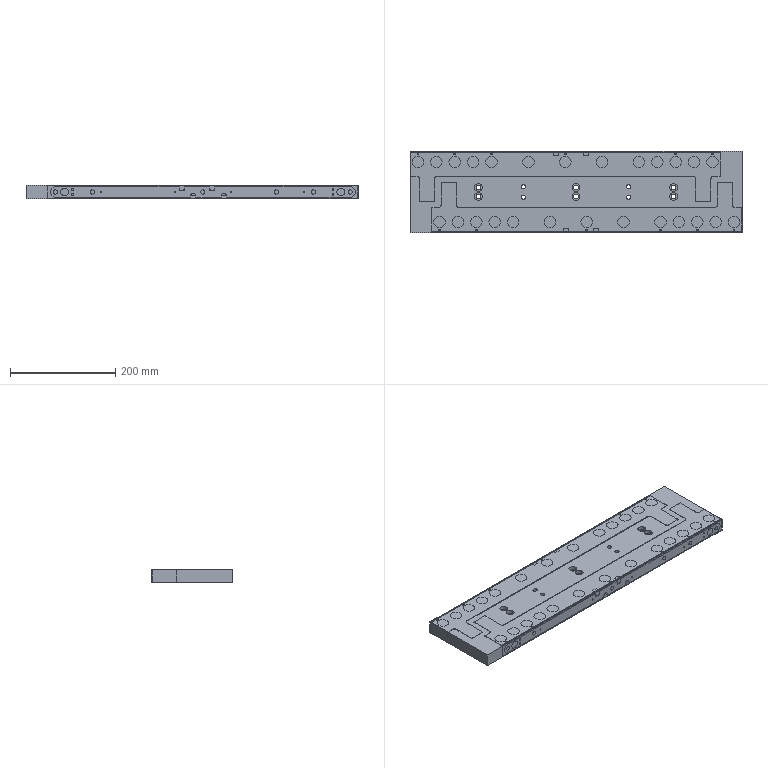NC program | NX | posted with a generic post | part box 631 x 154 x 25 mm
Whole program:
N10 G17 G21 G94 G90
(DRILLING_COPY_1_COPY , TOOL : D6A45)
N12 T07 M6
N14 G54
N16 G17 G0 G90 X280. Y0. B0. C0. S3000 M3
N18 G43 Z30. H7
N20 G94 G81 G98 Z-2.1 F200. R3.
N22 X262.5
N24 X247.5 Y-4.5
N26 Y4.5
N28 X210. Y0.
N30 X0.
N32 X-140.
N34 X-210.
N36 X-247.5 Y4.5
N38 Y-4.5
N40 X-262.5 Y0.
N42 X-280.
N44 G80
N46 G0 X-280. Y0. Z30.
(DRILLING_COPY_1_COPY_COPY , TOOL : D6A45)
N48 X-193.
N50 G81 Z-1.6 F200. R3.
N52 X-53.
N54 X53.
N56 X193.
N58 G80
N60 G0 X193. Y0. Z30.
N62 M5
(DRILLING_COPY_2_COPY_1 , TOOL : 3.3ZT)
N64 T13 M6
N66 G54
N68 G17 G0 G90 X-247.5 Y-4.5 B0. C0. S2000 M3
N70 G43 Z30. H13
N72 G94 G83 G98 Z-10.991 F100. Q2. R3.
N74 Y4.5
N76 X247.5
N78 Y-4.5
N80 G80
N82 G0 X247.5 Y-4.5 Z30.
N84 M5
(DRILLING_COPY_2_COPY_1_COPY , TOOL : 2.5ZT)
N86 T12 M6
N88 G54
N90 G17 G0 G90 X-193. Y0. B0. C0. S2000 M3
N92 G43 Z30. H12
N94 G94 G83 G98 Z-10.751 F100. Q2. R3.
N96 X-53.
N98 X53.
N100 X193.
N102 G80
N104 G0 X193. Y0. Z30.
N106 M5
(DRILLING_COPY_2_COPY_1_COPY_COPY , TOOL : 5.5ZT)
N108 T15 M6
N110 G54
N112 G17 G0 G90 X-40. Y7.5 B0. C0. S2000 M3
N114 G43 Z30. H15
N116 G94 G83 G98 Z-51.152 F250. Q2. R3.
N118 X-18. Y-7.5
N120 X18. Y7.5
N122 X40. Y-7.5
N124 G80
N126 G0 X40. Y-7.5 Z30.
N128 M5
(DRILLING_COPY_COPY_1 , TOOL : 10.5ZT)
N130 T09 M6
N132 G54
N134 G17 G0 G90 X-262.5 Y0. B0. C0. S1000 M3
N136 G43 Z30. H9
N138 G94 G83 G98 Z-99.204 F100. Q2. R3.
N140 X262.5
N142 G80
N144 G0 X262.5 Y0. Z30.
N146 M5
(DRILLING_COPY_COPY_COPY_1 , TOOL : 7.8ZT)
N148 T17 M6
N150 G54
N152 G17 G0 G90 X-280. Y0. B0. C0. S2000 M3
N154 G43 Z30. H17
N156 G94 G83 G98 Z-16.915 F200. Q2. R3.
N158 X-210.
N160 X-140.
N162 X0.
N164 X210.
N166 X280.
N168 G80
N170 G0 X280. Y0. Z30.
N172 M5
(DRILLING_COPY_COPY_COPY_COPY , TOOL : 8.0JD)
N174 T18 M6
N176 G54
N178 G17 G0 G90 X-280. Y0. B0. C0. S1000 M3
N180 G43 Z30. H18
N182 G94 G85 G98 Z-13.572 F50. R3.
N184 X-210.
N186 X-140.
N188 X0.
N190 X210.
N192 X280.
N194 G80
N196 G0 X280. Y0. Z30.
N198 M5
(HOLE_MILLING_COPY_1_COPY , TOOL : D10)
N200 T10 M6
N202 G54
N204 G17 G0 G90 X-262.5 Y0. B0. C0. S7000 M3
N206 G43 Z30. H10
N208 Z1.
N210 G94 G3 X-263.745 Y1.245 R1.245 F1500.
N212 X-264.99 Y0. R1.245
N214 X-264.99 Y0. Z0. I2.49 J0.
N216 X-264.99 Y0. Z-1. I2.49 J0.
N218 X-264.99 Y0. Z-2. I2.49 J0.
N220 X-264.99 Y0. Z-3. I2.49 J0.
N222 X-264.99 Y0. Z-4. I2.49 J0.
N224 X-264.99 Y0. Z-5. I2.49 J0.
N226 X-264.99 Y0. Z-6. I2.49 J0.
N228 X-264.99 Y0. Z-7. I2.49 J0.
N230 X-264.99 Y0. Z-8. I2.49 J0.
N232 X-264.99 Y0. Z-9. I2.49 J0.
N234 X-264.99 Y0. Z-10. I2.49 J0.
N236 X-264.99 Y0. Z-11. I2.49 J0.
N238 X-264.99 Y0. Z-12. I2.49 J0.
N240 X-264.99 Y0. Z-13. I2.49 J0.
N242 X-264.99 Y0. Z-14. I2.49 J0.
N244 X-264.99 Y0. Z-15. I2.49 J0.
N246 X-264.99 Y0. Z-16. I2.49 J0.
N248 X-264.99 Y0. Z-17. I2.49 J0.
N250 X-264.99 Y0. Z-18. I2.49 J0.
N252 X-264.99 Y0. Z-19. I2.49 J0.
N254 X-264.99 Y0. Z-20. I2.49 J0.
N256 X-264.99 Y0. Z-21. I2.49 J0.
N258 X-264.99 Y0. Z-22. I2.49 J0.
N260 X-264.99 Y0. Z-23. I2.49 J0.
N262 X-264.99 Y0. Z-24. I2.49 J0.
N264 X-264.99 Y0. Z-25. I2.49 J0.
N266 X-264.99 Y0. Z-26. I2.49 J0.
N268 X-264.99 Y0. Z-27. I2.49 J0.
N270 X-264.99 Y0. Z-28. I2.49 J0.
N272 X-264.99 Y0. Z-29. I2.49 J0.
N274 X-264.99 Y0. Z-30. I2.49 J0.
N276 X-264.99 Y0. Z-31. I2.49 J0.
N278 X-264.99 Y0. Z-32. I2.49 J0.
N280 X-264.99 Y0. Z-33. I2.49 J0.
N282 X-264.99 Y0. Z-34. I2.49 J0.
N284 X-264.99 Y0. Z-35. I2.49 J0.
N286 X-262.5 Y-2.49 R2.49
N288 X-264.99 Y0. R-2.49
N290 X-263.745 Y-1.245 R1.245
N292 X-262.5 Y0. R1.245
N294 G0 Z30.
N296 X262.5
N298 Z1.
N300 G3 X261.255 Y1.245 R1.245
N302 X260.01 Y0. R1.245
N304 X260.01 Y0. Z0. I2.49 J0.
N306 X260.01 Y0. Z-1. I2.49 J0.
N308 X260.01 Y0. Z-2. I2.49 J0.
N310 X260.01 Y0. Z-3. I2.49 J0.
N312 X260.01 Y0. Z-4. I2.49 J0.
N314 X260.01 Y0. Z-5. I2.49 J0.
N316 X260.01 Y0. Z-6. I2.49 J0.
N318 X260.01 Y0. Z-7. I2.49 J0.
N320 X260.01 Y0. Z-8. I2.49 J0.
N322 X260.01 Y0. Z-9. I2.49 J0.
N324 X260.01 Y0. Z-10. I2.49 J0.
N326 X260.01 Y0. Z-11. I2.49 J0.
N328 X260.01 Y0. Z-12. I2.49 J0.
N330 X260.01 Y0. Z-13. I2.49 J0.
N332 X260.01 Y0. Z-14. I2.49 J0.
N334 X260.01 Y0. Z-15. I2.49 J0.
N336 X260.01 Y0. Z-16. I2.49 J0.
N338 X260.01 Y0. Z-17. I2.49 J0.
N340 X260.01 Y0. Z-18. I2.49 J0.
N342 X260.01 Y0. Z-19. I2.49 J0.
N344 X260.01 Y0. Z-20. I2.49 J0.
N346 X260.01 Y0. Z-21. I2.49 J0.
N348 X260.01 Y0. Z-22. I2.49 J0.
N350 X260.01 Y0. Z-23. I2.49 J0.
N352 X260.01 Y0. Z-24. I2.49 J0.
N354 X260.01 Y0. Z-25. I2.49 J0.
N356 X260.01 Y0. Z-26. I2.49 J0.
N358 X260.01 Y0. Z-27. I2.49 J0.
N360 X260.01 Y0. Z-28. I2.49 J0.
N362 X260.01 Y0. Z-29. I2.49 J0.
N364 X260.01 Y0. Z-30. I2.49 J0.
N366 X260.01 Y0. Z-31. I2.49 J0.
N368 X260.01 Y0. Z-32. I2.49 J0.
N370 X260.01 Y0. Z-33. I2.49 J0.
N372 X260.01 Y0. Z-34. I2.49 J0.
N374 X260.01 Y0. Z-35. I2.49 J0.
N376 X262.5 Y-2.49 R2.49
N378 X260.01 Y0. R-2.49
N380 X261.255 Y-1.245 R1.245
N382 X262.5 Y0. R1.245
N384 G0 Z30.
(ZLEVEL_PROFILE_COPY_1 , TOOL : D10)
N386 X104.274 Y15.15
N388 Z1.5
N390 G1 X151.5 Z-0.975 F1000.
N392 X280. F3000.
N394 G2 X295.15 Y0. R15.15
N396 X280. Y-15.15 R15.15
N398 G1 X45.
N400 G2 X40. Y-11.234 R5.15
N402 X35. Y-15.15 R5.15
N404 G1 X-13.
N406 G2 X-18. Y-11.234 R5.15
N408 X-23. Y-15.15 R5.15
N410 G1 X-280.
N412 G2 X-295.15 Y0. R15.15
N414 X-280. Y15.15 R15.15
N416 G1 X-45.
N418 G2 X-40.018 Y11.306 R5.15
N420 G1 X-39.992 Y11.266
N422 G2 X-35. Y15.15 R5.15
N424 G1 X13.
N426 G2 X17.978 Y11.318 R5.15
N428 X23. Y15.15 R5.15
N430 G1 X151.5
N432 X207.358 Z-1.95
N434 X280.
N436 G2 X295.15 Y0. R15.15
N438 X280. Y-15.15 R15.15
N440 G1 X45.
N442 G2 X40. Y-11.234 R5.15
N444 X35. Y-15.15 R5.15
N446 G1 X-13.
N448 G2 X-18. Y-11.234 R5.15
N450 X-23. Y-15.15 R5.15
N452 G1 X-280.
N454 G2 X-295.15 Y0. R15.15
N456 X-280. Y15.15 R15.15
N458 G1 X-45.
N460 G2 X-40.018 Y11.306 R5.15
N462 G1 X-39.992 Y11.266
N464 G2 X-35. Y15.15 R5.15
N466 G1 X13.
N468 G2 X17.978 Y11.318 R5.15
N470 X23. Y15.15 R5.15
N472 G1 X207.358
N474 Z-0.45
N476 G0 Z30.
N478 M5
(HOLE_MILLING_COPY_1_COPY_COPY , TOOL : D10JING)
N480 T11 M6
N482 G54
N484 G17 G0 G90 X-262.5 Y0. B0. C0. S7000 M3
N486 G43 Z30. H11
N488 Z1.
N490 G94 G3 X-263.75 Y1.25 R1.25 F1000.
N492 X-265. Y0. R1.25
N494 X-265. Y0. Z-4. I2.5 J0.
N496 X-265. Y0. Z-9. I2.5 J0.
N498 X-265. Y0. Z-14. I2.5 J0.
N500 X-265. Y0. Z-19. I2.5 J0.
N502 X-265. Y0. Z-24. I2.5 J0.
N504 X-265. Y0. Z-29. I2.5 J0.
N506 X-265. Y0. Z-34. I2.5 J0.
N508 X-263.273 Y-2.378 Z-35. R2.5
N510 X-260.122 Y-0.773 R2.5
N512 X-263.273 Y-2.378 R-2.5
N514 X-261.697 Y-1.575 R1.25
N516 X-262.5 Y0. R1.25
N518 G0 Z30.
N520 X262.5
N522 Z1.
N524 G3 X261.25 Y1.25 R1.25
N526 X260. Y0. R1.25
N528 X260. Y0. Z-4. I2.5 J0.
N530 X260. Y0. Z-9. I2.5 J0.
N532 X260. Y0. Z-14. I2.5 J0.
N534 X260. Y0. Z-19. I2.5 J0.
N536 X260. Y0. Z-24. I2.5 J0.
N538 X260. Y0. Z-29. I2.5 J0.
N540 X260. Y0. Z-34. I2.5 J0.
N542 X261.727 Y-2.378 Z-35. R2.5
N544 X264.878 Y-0.773 R2.5
N546 X261.727 Y-2.378 R-2.5
N548 X263.303 Y-1.575 R1.25
N550 X262.5 Y0. R1.25
N552 G0 Z30.
(ZLEVEL_PROFILE_COPY_2 , TOOL : D10JING)
N554 X149.116 Y19.
N556 Z-2.
N558 G1 X149.53 Y16.653 F1200.
N560 G3 X151.5 Y15. R2.
N562 G1 X280.
N564 G2 X295. Y0. R15.
N566 X280. Y-15. R15.
N568 G1 X45.
N570 G2 X40.047 Y-10.682 R5.
N572 X35. Y-15. R5.
N574 G1 X-13.
N576 G2 X-17.99 Y-10.312 R5.
N578 G1 X-18.013 Y-10.315
N580 X-18.011 Y-10.337
N582 G2 X-23. Y-15. R5.
N584 G1 X-280.
N586 G2 X-295. Y0. R15.
N588 X-280. Y15. R15.
N590 G1 X-45.
N592 G2 X-40.047 Y10.682 R5.
N594 X-35. Y15. R5.
N596 G1 X13.
N598 G2 X17.989 Y10.326 R5.
N600 G1 X18.014 Y10.397
N602 X18.017 Y10.411
N604 G2 X23. Y15. R5.
N606 G1 X151.5
N608 G3 X153.47 Y16.653 R2.
N610 G1 X153.884 Y19.
N612 G0 Z30.
N614 M5
(111 , TOOL : D8JING)
N616 T08 M6
N618 G54
N620 G17 G0 G90 X17.999 Y19.413 B0. C0. S7000 M3
N622 G43 Z30. H8
N624 Z0.
N626 G94 G1 Z-1. F1800.
N628 X17.394 Y17.224
N630 G3 X16.998 Y16.529 R0.8
N632 G1 X17.001 Y16.131
N634 X17. Y10.
N636 Y7.5
N638 G3 X18. Y6.5 R1.
N640 X19. Y7.5 R1.
N642 G1 Y10.
N644 X19.003 Y16.529
N646 G3 X18.603 Y17.222 R0.8
N648 G1 X17.999 Y19.413
N650 Z0.
N652 G0 X18. Y19.411 Z-1.
N654 G1 Z-2.
N656 X17.394 Y17.224
N658 G3 X16.998 Y16.529 R0.8
N660 G1 X17.001 Y16.131
N662 X17. Y10.
N664 Y7.5
N666 G3 X18. Y6.5 R1.
N668 X19. Y7.5 R1.
N670 G1 Y10.
N672 X19.003 Y16.529
N674 G3 X18.603 Y17.222 R0.8
N676 G1 X18. Y19.411
N678 Z-1.
N680 G0 X18.001 Y19.414 Z-2.
N682 G1 Z-3.
N684 X17.394 Y17.224
N686 G3 X16.998 Y16.529 R0.8
N688 G1 X17.001 Y16.131
N690 Y12.546
N692 X17. Y12.148
N694 Y7.5
N696 G3 X18. Y6.5 R1.
N698 X19. Y7.5 R1.
N700 G1 Y12.148
N702 X19.003 Y16.529
N704 G3 X18.603 Y17.222 R0.8
N706 G1 X18.001 Y19.414
N708 Z-2.
N710 G0 Z-3.
N712 G1 Z-4.
N714 X17.394 Y17.224
N716 G3 X16.999 Y16.529 R0.8
N718 G1 X17.001 Y16.131
N720 Y12.546
N722 X17. Y12.148
N724 Y7.5
N726 G3 X18. Y6.5 R1.
N728 X19. Y7.5 R1.
N730 G1 Y12.148
N732 X19.003 Y16.529
N734 G3 X18.603 Y17.222 R0.8
N736 G1 X18.001 Y19.414
N738 Z-3.
N740 G0 Z-4.
N742 G1 Z-5.
N744 X17.394 Y17.224
N746 G3 X16.999 Y16.529 R0.8
N748 G1 X17.001 Y16.131
N750 Y12.546
N752 X17. Y12.148
N754 Y7.5
N756 G3 X18. Y6.5 R1.
N758 X19. Y7.5 R1.
N760 G1 Y12.148
N762 X19.002 Y16.529
N764 G3 X18.603 Y17.222 R0.8
N766 G1 X18.001 Y19.414
N768 Z-4.
N770 G0 Y19.415 Z-5.
N772 G1 Z-6.
N774 X17.394 Y17.224
N776 G3 X16.999 Y16.529 R0.8
N778 G1 X17.002 Y16.131
N780 Y12.546
N782 X17. Y12.148
N784 Y7.5
N786 G3 X18. Y6.5 R1.
N788 X19. Y7.5 R1.
N790 G1 Y12.148
N792 X19.002 Y16.529
N794 G3 X18.603 Y17.222 R0.8
N796 G1 X18.001 Y19.415
N798 Z-5.
N800 G0 Z-6.
N802 G1 Z-7.
N804 X17.394 Y17.224
N806 G3 X16.999 Y16.529 R0.8
N808 G1 X17.002 Y16.131
N810 Y12.546
N812 X17. Y12.148
N814 Y7.5
N816 G3 X18. Y6.5 R1.
N818 X19. Y7.5 R1.
N820 G1 Y12.148
N822 X19.002 Y16.529
N824 G3 X18.602 Y17.222 R0.8
N826 G1 X18.001 Y19.415
N828 Z-6.
N830 G0 Y19.416 Z-7.
N832 G1 Z-8.
N834 X17.395 Y17.224
N836 G3 X16.999 Y16.529 R0.8
N838 G1 X17.002 Y16.131
N840 Y12.546
N842 X17. Y12.148
N844 Y7.5
N846 G3 X18. Y6.5 R1.
N848 X19. Y7.5 R1.
N850 G1 Y12.148
N852 X19.002 Y16.529
N854 G3 X18.602 Y17.222 R0.8
N856 G1 X18.001 Y19.416
N858 Z-7.
N860 G0 Z30.
N862 X40. Y-19.411
N864 Z0.
N866 G1 Z-1.
N868 X40.61 Y-17.225
N870 G3 X41.004 Y-16.529 R0.8
N872 G1 X41. Y-16.131
N874 Y-12.489
N876 Y-7.5
N878 G3 X40. Y-6.5 R1.
N880 X39. Y-7.5 R1.
N882 G1 Y-12.489
N884 X38.997 Y-16.529
N886 G3 X39.396 Y-17.222 R0.8
N888 G1 X40. Y-19.411
N890 Z0.
N892 G0 Y-19.412 Z-1.
N894 G1 Z-2.
N896 X40.61 Y-17.225
N898 G3 X41.004 Y-16.529 R0.8
N900 G1 X41. Y-16.131
N902 Y-12.489
N904 Y-7.5
N906 G3 X40. Y-6.5 R1.
N908 X39. Y-7.5 R1.
N910 G1 Y-12.489
N912 X38.997 Y-16.529
N914 G3 X39.397 Y-17.222 R0.8
N916 G1 X40. Y-19.412
N918 Z-1.
N920 G0 Y-19.416 Z-2.
N922 G1 Z-3.
N924 X40.604 Y-17.222
N926 G3 X41.003 Y-16.529 R0.8
N928 G1 X41. Y-12.489
N930 Y-7.5
N932 G3 X40. Y-6.5 R1.
N934 X39. Y-7.5 R1.
N936 G1 Y-12.489
N938 X39.001 Y-12.5
N940 X38.982 Y-12.88
N942 X39.001 Y-12.895
N944 Y-16.131
N946 X38.998 Y-16.529
N948 G3 X39.392 Y-17.225 R0.8
N950 G1 X40. Y-19.416
N952 Z-2.
N954 G0 Z-3.
N956 G1 Z-4.
N958 X40.604 Y-17.222
N960 G3 X41.003 Y-16.529 R0.8
N962 G1 X41. Y-12.489
N964 Y-7.5
N966 G3 X40. Y-6.5 R1.
N968 X39. Y-7.5 R1.
N970 G1 Y-12.489
N972 X39.001 Y-12.5
N974 X38.982 Y-12.88
N976 X39.001 Y-12.895
N978 Y-16.131
N980 X38.998 Y-16.529
N982 G3 X39.392 Y-17.225 R0.8
N984 G1 X40. Y-19.416
N986 Z-3.
N988 G0 Y-19.417 Z-4.
N990 G1 Z-5.
N992 X40.604 Y-17.222
N994 G3 X41.003 Y-16.529 R0.8
N996 G1 X41. Y-12.489
N998 Y-7.5
N1000 G3 X40. Y-6.5 R1.
N1002 X39. Y-7.5 R1.
N1004 G1 Y-12.489
N1006 X39.001 Y-12.5
N1008 X38.982 Y-12.88
N1010 X39.001 Y-12.895
N1012 Y-16.131
N1014 X38.998 Y-16.529
N1016 G3 X39.392 Y-17.225 R0.8
N1018 G1 X40. Y-19.417
N1020 Z-4.
N1022 G0 Z-5.
N1024 G1 Z-6.
N1026 X40.604 Y-17.222
N1028 G3 X41.003 Y-16.529 R0.8
N1030 G1 X41. Y-12.489
N1032 Y-7.5
N1034 G3 X40. Y-6.5 R1.
N1036 X39. Y-7.5 R1.
N1038 G1 Y-12.489
N1040 X39.002 Y-12.5
N1042 X38.982 Y-12.88
N1044 X39.002 Y-12.895
N1046 X39.001 Y-16.131
N1048 X38.998 Y-16.529
N1050 G3 X39.393 Y-17.225 R0.8
N1052 G1 X40. Y-19.417
N1054 Z-5.
N1056 G0 X40.001 Z-6.
N1058 G1 Z-7.
N1060 X40.61 Y-17.226
N1062 G3 X41.003 Y-16.529 R0.8
N1064 G1 X40.999 Y-16.131
N1066 X41. Y-12.489
N1068 Y-7.5
N1070 G3 X40. Y-6.5 R1.
N1072 X39. Y-7.5 R1.
N1074 G1 Y-12.489
N1076 X39.002 Y-12.5
N1078 X38.982 Y-12.88
N1080 X39.002 Y-12.895
N1082 Y-16.131
N1084 X38.999 Y-16.529
N1086 G3 X39.393 Y-17.225 R0.8
N1088 G1 X40.001 Y-19.417
N1090 Z-6.
N1092 G0 X40. Y-19.418 Z-7.
N1094 G1 Z-8.
N1096 X40.603 Y-17.222
N1098 G3 X41.003 Y-16.529 R0.8
N1100 G1 X41. Y-12.489
N1102 Y-7.5
N1104 G3 X40. Y-6.5 R1.
N1106 X39. Y-7.5 R1.
N1108 G1 Y-12.489
N1110 X39.002 Y-12.5
N1112 X38.983 Y-12.868
N1114 X39.002 Y-12.882
N1116 Y-16.131
N1118 X38.999 Y-16.529
N1120 G3 X39.393 Y-17.225 R0.8
N1122 G1 X40. Y-19.418
N1124 Z-7.
N1126 G0 Z30.
N1128 X-17.999 Y-19.411
N1130 Z0.
N1132 G1 Z-1.
N1134 X-17.393 Y-17.224
N1136 G3 X-16.998 Y-16.529 R0.8
N1138 G1 X-17. Y-16.131
N1140 Y-12.489
N1142 Y-7.5
N1144 G3 X-18. Y-6.5 R1.
N1146 X-19. Y-7.5 R1.
N1148 G1 Y-12.489
N1150 X-19.003 Y-16.529
N1152 G3 X-18.603 Y-17.222 R0.8
N1154 G1 X-17.999 Y-19.411
N1156 Z0.
N1158 G0 Z-1.
N1160 G1 Z-2.
N1162 X-17.393 Y-17.224
N1164 G3 X-16.998 Y-16.529 R0.8
N1166 G1 X-17. Y-16.131
N1168 Y-12.489
N1170 Y-7.5
N1172 G3 X-18. Y-6.5 R1.
N1174 X-19. Y-7.5 R1.
N1176 G1 Y-12.489
N1178 X-19.003 Y-16.529
N1180 G3 X-18.603 Y-17.222 R0.8
N1182 G1 X-17.999 Y-19.411
N1184 Z-1.
N1186 G0 X-18. Y-19.414 Z-2.
N1188 G1 Z-3.
N1190 X-17.393 Y-17.225
N1192 G3 X-16.998 Y-16.529 R0.8
N1194 G1 X-17.001 Y-16.131
N1196 X-17. Y-12.489
N1198 Y-7.5
N1200 G3 X-18. Y-6.5 R1.
N1202 X-19. Y-7.5 R1.
N1204 G1 X-18.999 Y-12.5
N1206 X-19.018 Y-12.88
N1208 X-18.999 Y-12.895
N1210 X-19. Y-16.131
N1212 X-19.002 Y-16.529
N1214 G3 X-18.607 Y-17.224 R0.8
N1216 G1 X-18. Y-19.414
N1218 Z-2.
N1220 G0 Z-3.
N1222 G1 Z-4.
N1224 X-17.393 Y-17.225
N1226 G3 X-16.998 Y-16.529 R0.8
N1228 G1 X-17.001 Y-16.131
N1230 X-17. Y-12.489
N1232 Y-7.5
N1234 G3 X-18. Y-6.5 R1.
N1236 X-19. Y-7.5 R1.
N1238 G1 X-18.999 Y-12.5
N1240 X-19.018 Y-12.88
N1242 X-18.999 Y-12.895
N1244 X-19. Y-16.131
N1246 X-19.002 Y-16.529
N1248 G3 X-18.606 Y-17.224 R0.8
N1250 G1 X-18. Y-19.414
N1252 Z-3.
N1254 G0 Y-19.415 Z-4.
N1256 G1 Z-5.
N1258 X-17.393 Y-17.225
N1260 G3 X-16.998 Y-16.529 R0.8
N1262 G1 X-17.001 Y-16.131
N1264 X-17. Y-12.489
N1266 Y-7.5
N1268 G3 X-18. Y-6.5 R1.
N1270 X-19. Y-7.5 R1.
N1272 G1 X-18.999 Y-12.5
N1274 X-19.018 Y-12.88
N1276 X-18.999 Y-12.895
N1278 Y-16.131
N1280 X-19.002 Y-16.529
N1282 G3 X-18.606 Y-17.224 R0.8
N1284 G1 X-18. Y-19.415
N1286 Z-4.
N1288 G0 Z-5.
N1290 G1 Z-6.
N1292 X-17.393 Y-17.225
N1294 G3 X-16.998 Y-16.529 R0.8
N1296 G1 X-17.001 Y-16.131
N1298 X-17. Y-12.489
N1300 Y-7.5
N1302 G3 X-18. Y-6.5 R1.
N1304 X-19. Y-7.5 R1.
N1306 G1 Y-12.489
N1308 X-18.999 Y-12.5
N1310 X-19.018 Y-12.88
N1312 X-18.999 Y-12.895
N1314 Y-16.131
N1316 X-19.002 Y-16.529
N1318 G3 X-18.606 Y-17.224 R0.8
N1320 G1 X-18. Y-19.415
N1322 Z-5.
N1324 G0 Z-6.
N1326 G1 Z-7.
N1328 X-17.393 Y-17.225
N1330 G3 X-16.999 Y-16.529 R0.8
N1332 G1 X-17.002 Y-16.131
N1334 X-17. Y-12.489
N1336 Y-7.5
N1338 G3 X-18. Y-6.5 R1.
N1340 X-19. Y-7.5 R1.
N1342 G1 Y-12.489
N1344 X-18.999 Y-12.5
N1346 X-19.018 Y-12.88
N1348 X-18.999 Y-12.895
N1350 Y-16.131
N1352 X-19.001 Y-16.529
N1354 G3 X-18.606 Y-17.224 R0.8
N1356 G1 X-18. Y-19.415
N1358 Z-6.
N1360 G0 Y-19.416 Z-7.
N1362 G1 Z-8.
N1364 X-17.393 Y-17.225
N1366 G3 X-16.999 Y-16.529 R0.8
N1368 G1 X-17.002 Y-16.131
N1370 X-17. Y-12.489
N1372 Y-7.5
N1374 G3 X-18. Y-6.5 R1.
N1376 X-19. Y-7.5 R1.
N1378 G1 Y-12.489
N1380 X-18.999 Y-12.5
N1382 X-19.018 Y-12.88
N1384 X-18.999 Y-12.895
N1386 Y-16.131
N1388 X-19.001 Y-16.529
N1390 G3 X-18.605 Y-17.224 R0.8
N1392 G1 X-18. Y-19.416
N1394 Z-7.
N1396 G0 Z30.
N1398 X-40.003 Y19.416
N1400 Z0.
N1402 G1 Z-1.
N1404 X-40.607 Y17.224
N1406 G3 X-41.004 Y16.529 R0.8
N1408 G1 X-41.002 Y16.131
N1410 X-41.001 Y10.156
N1412 X-41. Y10.
N1414 Y7.5
N1416 G3 X-40. Y6.5 R1.
N1418 X-39. Y7.5 R1.
N1420 G1 Y10.
N1422 X-38.997 Y16.728
N1424 G3 X-39.397 Y17.421 R0.8
N1426 G1 X-40.003 Y19.416
N1428 Z0.
N1430 G0 Z-1.
N1432 G1 Z-2.
N1434 X-40.607 Y17.224
N1436 G3 X-41.003 Y16.529 R0.8
N1438 G1 X-41.001 Y16.131
N1440 Y10.156
N1442 X-41. Y10.
N1444 Y7.5
N1446 G3 X-40. Y6.5 R1.
N1448 X-39. Y7.5 R1.
N1450 G1 Y10.
N1452 X-38.997 Y16.728
N1454 G3 X-39.397 Y17.421 R0.8
N1456 G1 X-40.003 Y19.416
N1458 Z-1.
N1460 G0 X-40.002 Z-2.
N1462 G1 Z-3.
N1464 X-40.606 Y17.224
N1466 G3 X-41.003 Y16.529 R0.8
N1468 G1 X-41.001 Y16.131
N1470 X-41. Y12.148
N1472 Y7.5
N1474 G3 X-40. Y6.5 R1.
N1476 X-39. Y7.5 R1.
N1478 G1 Y12.148
N1480 X-38.997 Y16.728
N1482 G3 X-39.397 Y17.421 R0.8
N1484 G1 X-40.002 Y19.416
N1486 Z-2.
N1488 G0 Z-3.
N1490 G1 Z-4.
N1492 X-40.606 Y17.224
N1494 G3 X-41.003 Y16.529 R0.8
N1496 G1 X-41.001 Y16.131
N1498 X-41. Y12.148
N1500 Y7.5
N1502 G3 X-40. Y6.5 R1.
N1504 X-39. Y7.5 R1.
N1506 G1 Y12.148
N1508 X-38.998 Y16.728
N1510 G3 X-39.397 Y17.421 R0.8
N1512 G1 X-40.002 Y19.416
N1514 Z-3.
N1516 G0 Y19.417 Z-4.
N1518 G1 Z-5.
N1520 X-40.605 Y17.224
N1522 G3 X-41.002 Y16.529 R0.8
N1524 G1 X-41.001 Y16.131
N1526 X-41. Y12.148
N1528 Y7.5
N1530 G3 X-40. Y6.5 R1.
N1532 X-39. Y7.5 R1.
N1534 G1 Y12.148
N1536 X-38.998 Y16.728
N1538 G3 X-39.397 Y17.421 R0.8
N1540 G1 X-40.002 Y19.417
N1542 Z-4.
N1544 G0 Z-5.
N1546 G1 Z-6.
N1548 X-40.605 Y17.224
N1550 G3 X-41.002 Y16.529 R0.8
N1552 G1 X-41. Y16.131
N1554 Y12.148
N1556 Y7.5
N1558 G3 X-40. Y6.5 R1.
N1560 X-39. Y7.5 R1.
N1562 G1 Y12.148
N1564 X-38.998 Y16.728
N1566 G3 X-39.397 Y17.421 R0.8
N1568 G1 X-40.002 Y19.417
N1570 Z-5.
N1572 G0 Y19.418 Z-6.
N1574 G1 Z-7.
N1576 X-40.605 Y17.223
N1578 G3 X-41.002 Y16.529 R0.8
N1580 G1 X-41. Y16.131
N1582 Y12.148
N1584 Y7.5
N1586 G3 X-40. Y6.5 R1.
N1588 X-39. Y7.5 R1.
N1590 G1 Y12.148
N1592 X-38.998 Y16.728
N1594 G3 X-39.398 Y17.421 R0.8
N1596 G1 X-40.002 Y19.418
N1598 Z-6.
N1600 G0 Z-7.
N1602 G1 Z-8.
N1604 X-40.604 Y17.223
N1606 G3 X-41.001 Y16.529 R0.8
N1608 G1 X-41. Y16.131
N1610 Y12.148
N1612 Y7.5
N1614 G3 X-40. Y6.5 R1.
N1616 X-39. Y7.5 R1.
N1618 G1 Y12.148
N1620 X-38.998 Y16.728
N1622 G3 X-39.398 Y17.421 R0.8
N1624 G1 X-40.002 Y19.418
N1626 Z-7.
N1628 G0 Z30.
N1630 M5
(ZLEVEL_PROFILE_COPY_1_COPY_COPY_COPY_COPY_2_COPY_COPY , TOOL : D6A45)
N1632 T07 M6
N1634 G54
N1636 G17 G0 G90 X278.561 Y-1.149 B0. C0. S7000 M3
N1638 G43 Z30. H7
N1640 Z-1.
N1642 G94 G1 X279.48 Y-2.741 F1000.
N1644 G3 X280. Y-3.041 R0.6
N1646 X283.041 Y0. R3.041
N1648 X280. Y-3.041 R-3.041
N1650 X280.52 Y-2.741 R0.6
N1652 G1 X281.439 Y-1.149
N1654 G0 Z30.
N1656 X208.561
N1658 Z-1.
N1660 G1 X209.48 Y-2.741
N1662 G3 X210. Y-3.041 R0.6
N1664 G1 X210.002
N1666 G3 X213.041 Y0.002 R3.041
N1668 X210. Y-3.041 R-3.041
N1670 X210.52 Y-2.741 R0.6
N1672 G1 X211.439 Y-1.149
N1674 G0 Z30.
N1676 X-1.439
N1678 Z-1.
N1680 G1 X-0.52 Y-2.741
N1682 G3 X0. Y-3.041 R0.6
N1684 G1 X0.003
N1686 G3 X3.041 Y0.003 R3.041
N1688 X0. Y-3.041 R-3.041
N1690 X0.52 Y-2.741 R0.6
N1692 G1 X1.439 Y-1.149
N1694 G0 Z30.
N1696 X-141.439
N1698 Z-1.
N1700 G1 X-140.52 Y-2.741
N1702 G3 X-140. Y-3.041 R0.6
N1704 X-136.959 Y0. R3.041
N1706 X-140. Y-3.041 R-3.041
N1708 X-139.48 Y-2.741 R0.6
N1710 G1 X-138.561 Y-1.149
N1712 G0 Z30.
N1714 X-211.439
N1716 Z-1.
N1718 G1 X-210.52 Y-2.741
N1720 G3 X-210. Y-3.041 R0.6
N1722 X-206.959 Y0. R3.041
N1724 X-210. Y-3.041 R-3.041
N1726 X-209.48 Y-2.741 R0.6
N1728 G1 X-208.561 Y-1.149
N1730 G0 Z30.
N1732 X263.606 Y5.226
N1734 Z-1.
N1736 G1 X263.02 Y6.241
N1738 G3 X262.5 Y6.541 R0.6
N1740 G1 X262.493
N1742 G3 X255.959 Y-0.007 R6.541
N1744 X262.5 Y6.541 R-6.541
N1746 X261.98 Y6.241 R0.6
N1748 G1 X261.394 Y5.226
N1750 G0 Z30.
N1752 X-261.394
N1754 Z-1.
N1756 G1 X-261.98 Y6.241
N1758 G3 X-262.5 Y6.541 R0.6
N1760 X-269.041 Y0. R6.541
N1762 X-262.5 Y6.541 R-6.541
N1764 X-263.02 Y6.241 R0.6
N1766 G1 X-263.606 Y5.226
N1768 G0 Z30.
N1770 X-278.561 Y1.149
N1772 Z-1.
N1774 G1 X-279.48 Y2.741
N1776 G3 X-280. Y3.041 R0.6
N1778 X-283.041 Y0. R3.041
N1780 X-280. Y3.041 R-3.041
N1782 X-280.52 Y2.741 R0.6
N1784 G1 X-281.439 Y1.149
N1786 G0 Z30.
N1788 X-22.079 Y-11.953
N1790 Z-1.
N1792 G1 X-22.48 Y-11.259
N1794 G3 X-22.999 Y-10.959 R0.6
N1796 G1 X-280.
N1798 G2 X-290.959 Y0. R10.959
N1800 X-280. Y10.959 R10.959
N1802 G1 X-44.999
N1804 G2 X-44.041 Y10.001 R0.958
N1806 G1 Y7.5
N1808 G3 X-40. Y3.459 R4.041
N1810 X-35.959 Y7.5 R4.041
N1812 G1 Y10.001
N1814 G2 X-35.001 Y10.959 R0.958
N1816 G1 X13.001
N1818 G2 X13.959 Y10.001 R0.958
N1820 G1 Y7.5
N1822 G3 X18. Y3.459 R4.041
N1824 X22.041 Y7.5 R4.041
N1826 G1 Y10.001
N1828 G2 X22.999 Y10.959 R0.958
N1830 G1 X280.
N1832 G2 X290.959 Y0. R10.959
N1834 X280. Y-10.959 R10.959
N1836 G1 X44.999
N1838 G2 X44.041 Y-10.001 R0.958
N1840 G1 Y-7.5
N1842 G3 X40. Y-3.459 R4.041
N1844 X35.959 Y-7.5 R4.041
N1846 G1 Y-10.001
N1848 G2 X35.001 Y-10.959 R0.958
N1850 G1 X-13.001
N1852 G2 X-13.959 Y-10.001 R0.958
N1854 G1 Y-7.5
N1856 G3 X-18. Y-3.459 R4.041
N1858 X-22.041 Y-7.5 R4.041
N1860 G1 Y-10.001
N1862 G2 X-22.999 Y-10.959 R0.958
N1864 G3 X-23.519 Y-11.259 R0.6
N1866 G1 X-24.039 Y-12.159
N1868 G0 Z30.
(ZLEVEL_PROFILE_COPY_1_COPY_COPY_COPY_COPY_2_COPY_COPY_COPY , TOOL : D6A45)
N1870 X-38.984 Y11.33
N1872 Z-4.
N1874 G1 X-37.325 Y12.141
N1876 G3 X-36.99 Y12.639 R0.6
N1878 G2 X-35.001 Y14.5 R1.997
N1880 G1 X13.001
N1882 G2 X14.995 Y12.641 R2.006
N1884 G3 X15.332 Y12.145 R0.6
N1886 G1 X16.977 Y11.349
N1888 G0 Z30.
N1890 X19.411 Y12.182
N1892 Z-4.
N1894 G1 X20.676 Y12.368
N1896 G3 X21.146 Y12.74 R0.6
N1898 G2 X22.999 Y14. R1.996
N1900 G1 X294.501
N1902 G2 X296.5 Y12.001 R2.007
N1904 G1 Y-12.001
N1906 G2 X294.501 Y-14. R2.007
N1908 G1 X44.999
N1910 G2 X43.146 Y-12.741 R2.
N1912 G3 X42.674 Y-12.369 R0.6
N1914 G1 X41.414 Y-12.187
N1916 G0 Z30.
N1918 X38.589 Y-12.181
N1920 Z-4.
N1922 G1 X37.326 Y-12.366
N1924 G3 X36.855 Y-12.738 R0.6
N1926 G2 X35.001 Y-14. R2.
N1928 G1 X-13.001
N1930 G2 X-14.854 Y-12.74 R1.996
N1932 G3 X-15.324 Y-12.368 R0.6
N1934 G1 X-16.589 Y-12.182
N1936 G0 Z30.
N1938 X-19.423 Y-12.201
N1940 Z-4.
N1942 G1 X-20.672 Y-12.372
N1944 G3 X-21.146 Y-12.74 R0.6
N1946 G2 X-22.999 Y-14. R2.026
N1948 G1 X-294.501
N1950 G2 X-296.5 Y-12.001 R2.007
N1952 G1 Y12.001
N1954 G2 X-294.501 Y14. R2.007
N1956 G1 X-44.999
N1958 G2 X-43.146 Y12.741 R2.
N1960 G3 X-42.674 Y12.369 R0.6
N1962 G1 X-41.414 Y12.187
N1964 G0 Z30.
N1966 M5
N1968 M2